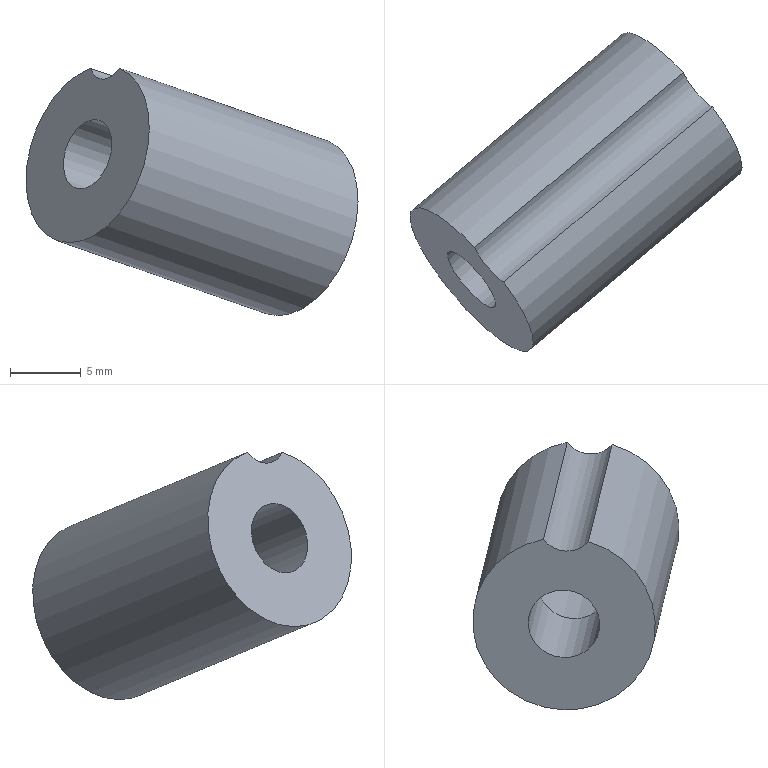Part | NX | features solid 2 | 1 solid | 7 faces | box 23.544 x 22.608 x 17.54 mm | volume 1782 mm3 | cylinder 4 | plane 3 | commonest cylinder face diameters 4 x1 5.1 x1 8.4 x1 13 x1
STEP:
#1=CARTESIAN_POINT('',(-605.494,-4.43,-13.594));
#2=VERTEX_POINT('',#1);
#3=CARTESIAN_POINT('',(-620.293,-16.848,-8.418));
#4=VERTEX_POINT('',#3);
#5=CARTESIAN_POINT('',(-612.893,-10.639,-11.006));
#6=DIRECTION('',(-0.7399,-0.6209,0.2588));
#7=VECTOR('',#6,1000.);
#8=LINE('',#5,#7);
#9=EDGE_CURVE('',#2,#4,#8,.T.);
#10=ORIENTED_EDGE('',*,*,#9,.F.);
#11=CARTESIAN_POINT('',(-603.437,-6.881,-13.594));
#12=VERTEX_POINT('',#11);
#13=CARTESIAN_POINT('',(-605.715,-6.704,-19.679));
#14=DIRECTION('',(-0.7399,-0.6209,0.2588));
#15=DIRECTION('',(0.1983,0.1664,0.9659));
#16=AXIS2_PLACEMENT_3D('',#13,#14,#15);
#17=CIRCLE('',#16,6.5);
#18=EDGE_CURVE('',#2,#12,#17,.T.);
#19=ORIENTED_EDGE('',*,*,#18,.T.);
#20=CARTESIAN_POINT('',(-618.236,-19.299,-8.418));
#21=VERTEX_POINT('',#20);
#22=CARTESIAN_POINT('',(-610.836,-13.09,-11.006));
#23=DIRECTION('',(-0.7399,-0.6209,0.2588));
#24=VECTOR('',#23,1000.);
#25=LINE('',#22,#24);
#26=EDGE_CURVE('',#21,#12,#25,.F.);
#27=ORIENTED_EDGE('',*,*,#26,.F.);
#28=CARTESIAN_POINT('',(-620.513,-19.121,-14.503));
#29=DIRECTION('',(-0.7399,-0.6209,0.2588));
#30=DIRECTION('',(0.1983,0.1664,0.9659));
#31=AXIS2_PLACEMENT_3D('',#28,#29,#30);
#32=CIRCLE('',#31,6.5);
#33=EDGE_CURVE('',#4,#21,#32,.T.);
#34=ORIENTED_EDGE('',*,*,#33,.F.);
#35=EDGE_LOOP('',(#10,#19,#27,#34));
#36=FACE_BOUND('',#35,.T.);
#37=CARTESIAN_POINT('',(-605.715,-6.704,-19.679));
#38=DIRECTION('',(-0.7399,-0.6209,0.2588));
#39=DIRECTION('',(0.1983,0.1664,0.9659));
#40=AXIS2_PLACEMENT_3D('',#37,#38,#39);
#41=CYLINDRICAL_SURFACE('',#40,6.5);
#42=ADVANCED_FACE('',(#36),#41,.T.);
#43=CARTESIAN_POINT('',(-604.882,-6.005,-15.622));
#44=VERTEX_POINT('',#43);
#45=CARTESIAN_POINT('',(-605.715,-6.704,-19.679));
#46=DIRECTION('',(-0.7399,-0.6209,0.2588));
#47=DIRECTION('',(0.1983,0.1664,0.9659));
#48=AXIS2_PLACEMENT_3D('',#45,#46,#47);
#49=CIRCLE('',#48,4.2);
#50=EDGE_CURVE('',#44,#44,#49,.T.);
#51=ORIENTED_EDGE('',*,*,#50,.T.);
#52=EDGE_LOOP('',(#51));
#53=FACE_BOUND('',#52,.T.);
#54=ORIENTED_EDGE('',*,*,#18,.F.);
#55=CARTESIAN_POINT('',(-604.228,-5.456,-12.435));
#56=DIRECTION('',(-0.7399,-0.6209,0.2588));
#57=DIRECTION('',(0.1983,0.1664,0.9659));
#58=AXIS2_PLACEMENT_3D('',#55,#56,#57);
#59=CIRCLE('',#58,2.);
#60=EDGE_CURVE('',#2,#12,#59,.T.);
#61=ORIENTED_EDGE('',*,*,#60,.T.);
#62=EDGE_LOOP('',(#54,#61));
#63=FACE_BOUND('',#62,.T.);
#64=CARTESIAN_POINT('',(-605.715,-6.704,-19.679));
#65=DIRECTION('',(-0.7399,-0.6209,0.2588));
#66=DIRECTION('',(0.1983,0.1664,0.9659));
#67=AXIS2_PLACEMENT_3D('',#64,#65,#66);
#68=PLANE('',#67);
#69=ADVANCED_FACE('',(#53,#63),#68,.F.);
#70=CARTESIAN_POINT('',(-620.008,-18.697,-12.04));
#71=VERTEX_POINT('',#70);
#72=CARTESIAN_POINT('',(-620.513,-19.121,-14.503));
#73=DIRECTION('',(-0.7399,-0.6209,0.2588));
#74=DIRECTION('',(0.1983,0.1664,0.9659));
#75=AXIS2_PLACEMENT_3D('',#72,#73,#74);
#76=CIRCLE('',#75,2.55);
#77=EDGE_CURVE('',#71,#71,#76,.T.);
#78=ORIENTED_EDGE('',*,*,#77,.F.);
#79=EDGE_LOOP('',(#78));
#80=FACE_BOUND('',#79,.T.);
#81=CARTESIAN_POINT('',(-619.026,-17.874,-7.259));
#82=DIRECTION('',(-0.7399,-0.6209,0.2588));
#83=DIRECTION('',(0.1983,0.1664,0.9659));
#84=AXIS2_PLACEMENT_3D('',#81,#82,#83);
#85=CIRCLE('',#84,2.);
#86=EDGE_CURVE('',#4,#21,#85,.T.);
#87=ORIENTED_EDGE('',*,*,#86,.F.);
#88=ORIENTED_EDGE('',*,*,#33,.T.);
#89=EDGE_LOOP('',(#87,#88));
#90=FACE_BOUND('',#89,.T.);
#91=CARTESIAN_POINT('',(-620.513,-19.121,-14.503));
#92=DIRECTION('',(-0.7399,-0.6209,0.2588));
#93=DIRECTION('',(0.1983,0.1664,0.9659));
#94=AXIS2_PLACEMENT_3D('',#91,#92,#93);
#95=PLANE('',#94);
#96=ADVANCED_FACE('',(#80,#90),#95,.T.);
#97=ORIENTED_EDGE('',*,*,#50,.F.);
#98=EDGE_LOOP('',(#97));
#99=FACE_BOUND('',#98,.T.);
#100=CARTESIAN_POINT('',(-613.761,-13.456,-12.517));
#101=VERTEX_POINT('',#100);
#102=CARTESIAN_POINT('',(-614.594,-14.154,-16.574));
#103=DIRECTION('',(-0.7399,-0.6209,0.2588));
#104=DIRECTION('',(0.1983,0.1664,0.9659));
#105=AXIS2_PLACEMENT_3D('',#102,#103,#104);
#106=CIRCLE('',#105,4.2);
#107=EDGE_CURVE('',#101,#101,#106,.T.);
#108=ORIENTED_EDGE('',*,*,#107,.T.);
#109=EDGE_LOOP('',(#108));
#110=FACE_BOUND('',#109,.T.);
#111=CARTESIAN_POINT('',(-605.715,-6.704,-19.679));
#112=DIRECTION('',(-0.7399,-0.6209,0.2588));
#113=DIRECTION('',(0.1983,0.1664,0.9659));
#114=AXIS2_PLACEMENT_3D('',#111,#112,#113);
#115=CYLINDRICAL_SURFACE('',#114,4.2);
#116=ADVANCED_FACE('',(#99,#110),#115,.F.);
#117=CARTESIAN_POINT('',(-614.088,-13.73,-14.11));
#118=VERTEX_POINT('',#117);
#119=CARTESIAN_POINT('',(-614.594,-14.154,-16.574));
#120=DIRECTION('',(-0.7399,-0.6209,0.2588));
#121=DIRECTION('',(0.1983,0.1664,0.9659));
#122=AXIS2_PLACEMENT_3D('',#119,#120,#121);
#123=CIRCLE('',#122,2.55);
#124=EDGE_CURVE('',#118,#118,#123,.T.);
#125=ORIENTED_EDGE('',*,*,#124,.T.);
#126=EDGE_LOOP('',(#125));
#127=FACE_BOUND('',#126,.T.);
#128=ORIENTED_EDGE('',*,*,#107,.F.);
#129=EDGE_LOOP('',(#128));
#130=FACE_BOUND('',#129,.T.);
#131=CARTESIAN_POINT('',(-614.594,-14.154,-16.574));
#132=DIRECTION('',(-0.7399,-0.6209,0.2588));
#133=DIRECTION('',(0.1983,0.1664,0.9659));
#134=AXIS2_PLACEMENT_3D('',#131,#132,#133);
#135=PLANE('',#134);
#136=ADVANCED_FACE('',(#127,#130),#135,.F.);
#137=ORIENTED_EDGE('',*,*,#9,.T.);
#138=ORIENTED_EDGE('',*,*,#86,.T.);
#139=ORIENTED_EDGE('',*,*,#26,.T.);
#140=ORIENTED_EDGE('',*,*,#60,.F.);
#141=EDGE_LOOP('',(#137,#138,#139,#140));
#142=FACE_BOUND('',#141,.T.);
#143=CARTESIAN_POINT('',(-604.228,-5.456,-12.435));
#144=DIRECTION('',(-0.7399,-0.6209,0.2588));
#145=DIRECTION('',(0.1983,0.1664,0.9659));
#146=AXIS2_PLACEMENT_3D('',#143,#144,#145);
#147=CYLINDRICAL_SURFACE('',#146,2.);
#148=ADVANCED_FACE('',(#142),#147,.F.);
#149=ORIENTED_EDGE('',*,*,#77,.T.);
#150=EDGE_LOOP('',(#149));
#151=FACE_BOUND('',#150,.T.);
#152=ORIENTED_EDGE('',*,*,#124,.F.);
#153=EDGE_LOOP('',(#152));
#154=FACE_BOUND('',#153,.T.);
#155=CARTESIAN_POINT('',(-605.715,-6.704,-19.679));
#156=DIRECTION('',(-0.7399,-0.6209,0.2588));
#157=DIRECTION('',(0.1983,0.1664,0.9659));
#158=AXIS2_PLACEMENT_3D('',#155,#156,#157);
#159=CYLINDRICAL_SURFACE('',#158,2.55);
#160=ADVANCED_FACE('',(#151,#154),#159,.F.);
#161=CLOSED_SHELL('',(#42,#69,#96,#116,#136,#148,#160));
#162=MANIFOLD_SOLID_BREP('',#161);
#163=(LENGTH_UNIT()NAMED_UNIT(*)SI_UNIT(.MILLI.,.METRE.));
#164=UNCERTAINTY_MEASURE_WITH_UNIT(LENGTH_MEASURE(0.00001),#163,'','');
#165=(NAMED_UNIT(*)PLANE_ANGLE_UNIT()SI_UNIT($,.RADIAN.));
#166=(NAMED_UNIT(*)SI_UNIT($,.STERADIAN.)SOLID_ANGLE_UNIT());
#167=(GEOMETRIC_REPRESENTATION_CONTEXT(3)GLOBAL_UNCERTAINTY_ASSIGNED_CONTEXT((#164))GLOBAL_UNIT_ASSIGNED_CONTEXT((#163,#165,#166))REPRESENTATION_CONTEXT('',''));
#168=ADVANCED_BREP_SHAPE_REPRESENTATION('',(#162),#167);